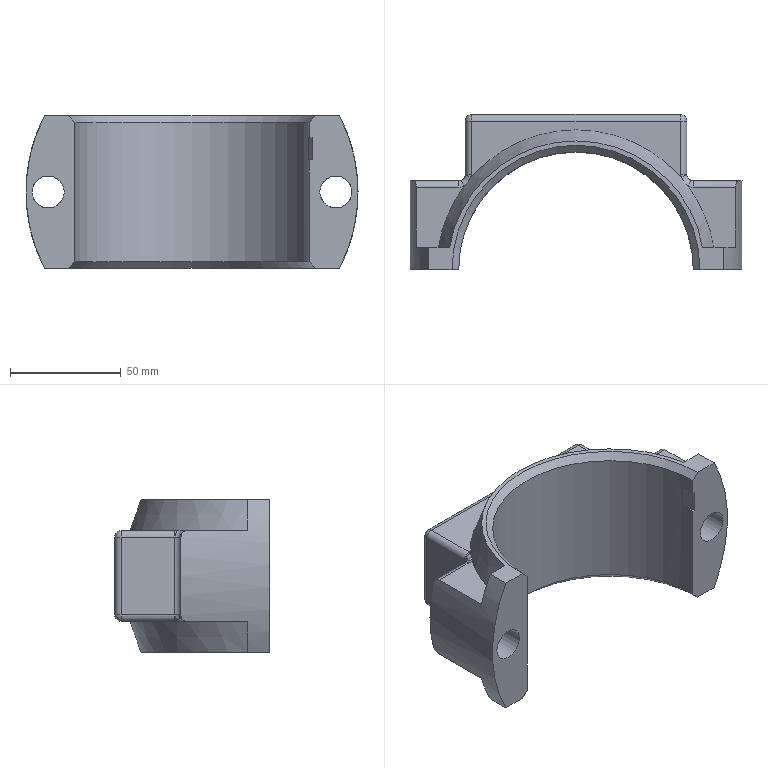Part | NX | features DATUM_CSYS 9, SKETCH 7, EXTRUDE 6, BLEND 2, CHAMFER 1, SWP104 1, UNITE 1 | 1 solid | 61 faces | box 150 x 70 x 69 mm | volume 212244 mm3 | plane 22 | cylinder 19 | torus 8 | cone 4 | spline 4 | sphere 4 | commonest cylinder face diameters 6 x14 14.5 x2 150 x2 106 x1